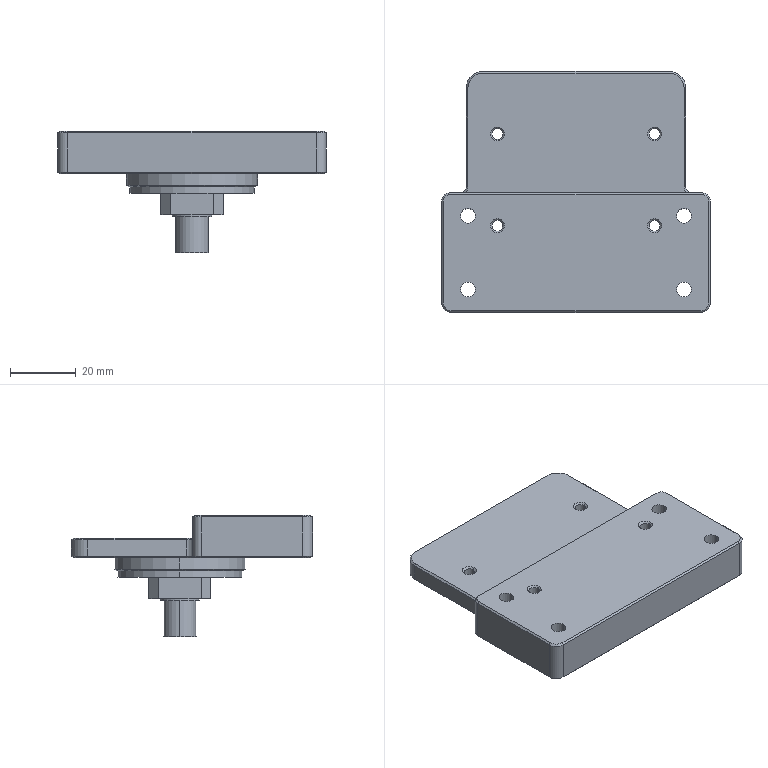Part | SolidWorks | features BaseBody 1 | 1 solid | 139 faces | box 82 x 73.6 x 37.1 mm | volume 61964 mm3 | cylinder 50 | plane 47 | cone 42 | commonest cylinder face diameters 3.3 x8 3.5 x8 4.5 x8 8 x8 10 x4 4 x2